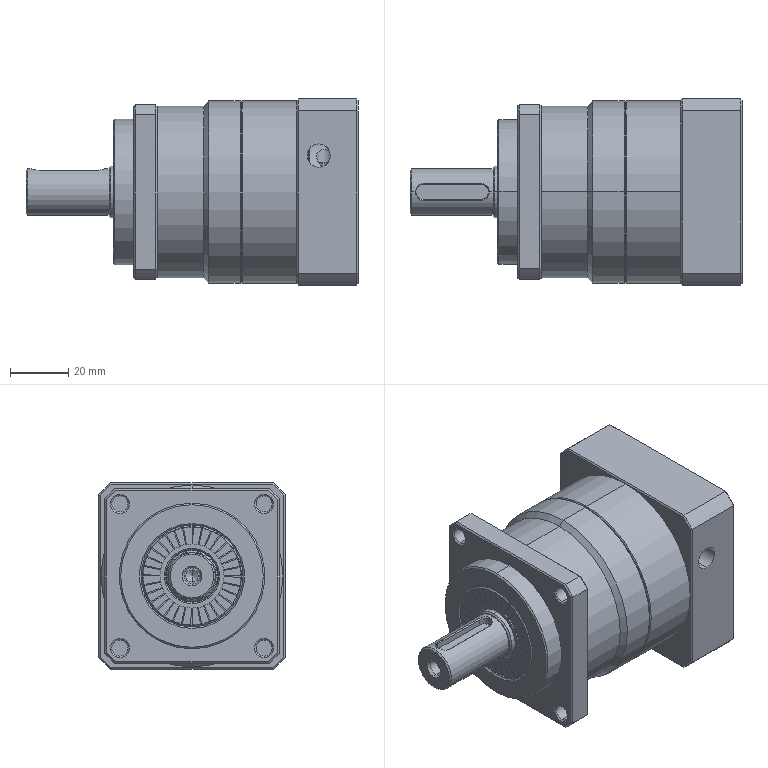Part | SolidWorks | features BaseBody 23 | 23 solids | 1216 faces | box 114 x 64 x 64 mm | volume 228770 mm3 | plane 423 | cylinder 354 | spline 244 | cone 195 | commonest cylinder face diameters 22 x34 3.3 x32 33.5 x32 4 x24 4.5 x24 7 x24